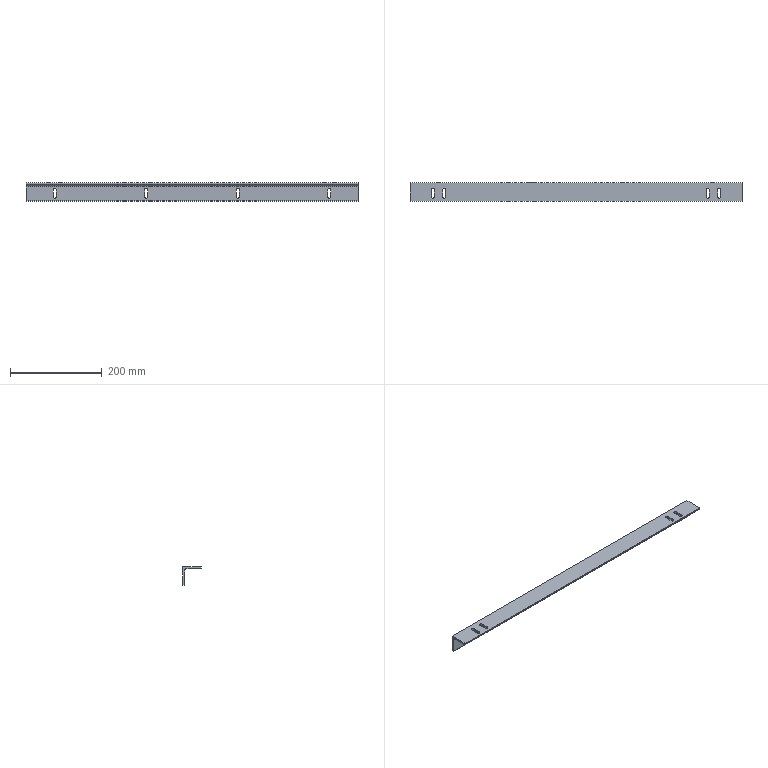Part | STEP file | PN_0015_angle steel_default_machined_ | 1 solid | 51 faces | box 725 x 40 x 40 mm | volume 219145 mm3 | cylinder 27 | plane 24 | commonest cylinder face diameters 7 x24 2.667 x2 10 x1